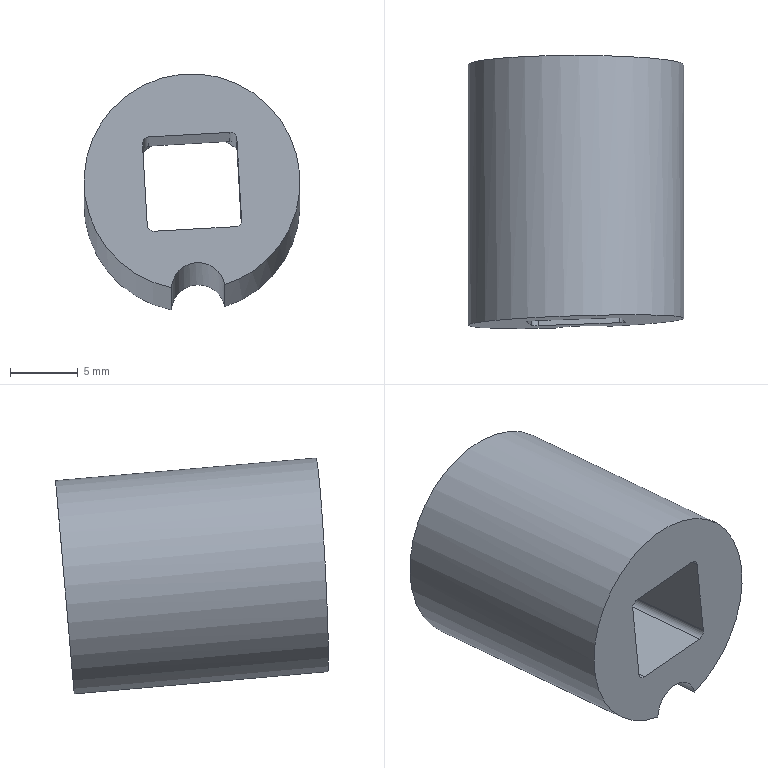Part | NX | features solid 2 | 1 solid | 14 faces | box 16 x 20.204 x 17.479 mm | volume 2341 mm3 | plane 7 | cylinder 7 | commonest cylinder face diameters 1 x4 4 x1 10.6 x1 16 x1
STEP:
#1=CARTESIAN_POINT('',(-229.897,-58.074,-39.843));
#2=VERTEX_POINT('',#1);
#3=CARTESIAN_POINT('',(-225.935,-57.934,-39.624));
#4=VERTEX_POINT('',#3);
#5=CARTESIAN_POINT('',(-227.901,-58.017,-39.983));
#6=DIRECTION('',(-0.03252,0.9981,-0.05307));
#7=DIRECTION('',(0.6892,-0.01607,-0.7244));
#8=AXIS2_PLACEMENT_3D('',#5,#6,#7);
#9=ELLIPSE('',#8,2.002,2.);
#10=EDGE_CURVE('',#2,#4,#9,.T.);
#11=ORIENTED_EDGE('',*,*,#10,.T.);
#12=CARTESIAN_POINT('',(-228.366,-57.608,-32.002));
#13=DIRECTION('',(-0.03252,0.9981,-0.05307));
#14=DIRECTION('',(0.6892,-0.01607,-0.7244));
#15=AXIS2_PLACEMENT_3D('',#12,#13,#14);
#16=ELLIPSE('',#15,8.009,8.);
#17=EDGE_CURVE('',#2,#4,#16,.T.);
#18=ORIENTED_EDGE('',*,*,#17,.F.);
#19=EDGE_LOOP('',(#11,#18));
#20=FACE_BOUND('',#19,.T.);
#21=CARTESIAN_POINT('',(-231.158,-57.893,-35.659));
#22=VERTEX_POINT('',#21);
#23=CARTESIAN_POINT('',(-225.168,-57.68,-35.328));
#24=VERTEX_POINT('',#23);
#25=CARTESIAN_POINT('',(-414.975,-64.423,-45.84));
#26=DIRECTION('',(-0.9978,-0.03545,-0.05527));
#27=VECTOR('',#26,1000.);
#28=LINE('',#25,#27);
#29=EDGE_CURVE('',#22,#24,#28,.F.);
#30=ORIENTED_EDGE('',*,*,#29,.F.);
#31=CARTESIAN_POINT('',(-231.686,-57.885,-35.188));
#32=VERTEX_POINT('',#31);
#33=CARTESIAN_POINT('',(-231.187,-57.867,-35.161));
#34=DIRECTION('',(-0.03252,0.9981,-0.05307));
#35=DIRECTION('',(-0.6892,0.01607,0.7244));
#36=AXIS2_PLACEMENT_3D('',#33,#34,#35);
#37=ELLIPSE('',#36,0.5006,0.5);
#38=EDGE_CURVE('',#22,#32,#37,.T.);
#39=ORIENTED_EDGE('',*,*,#38,.T.);
#40=CARTESIAN_POINT('',(-232.035,-57.578,-29.202));
#41=VERTEX_POINT('',#40);
#42=CARTESIAN_POINT('',(-239.027,-51.43,90.7));
#43=DIRECTION('',(0.05814,-0.05112,-0.997));
#44=VECTOR('',#43,1000.);
#45=LINE('',#42,#44);
#46=EDGE_CURVE('',#32,#41,#45,.F.);
#47=ORIENTED_EDGE('',*,*,#46,.T.);
#48=CARTESIAN_POINT('',(-231.565,-57.535,-28.676));
#49=VERTEX_POINT('',#48);
#50=CARTESIAN_POINT('',(-231.536,-57.561,-29.175));
#51=DIRECTION('',(-0.03252,0.9981,-0.05307));
#52=DIRECTION('',(0.6892,-0.01607,-0.7244));
#53=AXIS2_PLACEMENT_3D('',#50,#51,#52);
#54=ELLIPSE('',#53,0.5006,0.5);
#55=EDGE_CURVE('',#41,#49,#54,.T.);
#56=ORIENTED_EDGE('',*,*,#55,.T.);
#57=CARTESIAN_POINT('',(-225.575,-57.322,-28.344));
#58=VERTEX_POINT('',#57);
#59=CARTESIAN_POINT('',(-415.374,-64.065,-38.856));
#60=DIRECTION('',(-0.9978,-0.03545,-0.05527));
#61=VECTOR('',#60,1000.);
#62=LINE('',#59,#61);
#63=EDGE_CURVE('',#49,#58,#62,.F.);
#64=ORIENTED_EDGE('',*,*,#63,.T.);
#65=CARTESIAN_POINT('',(-225.047,-57.33,-28.815));
#66=VERTEX_POINT('',#65);
#67=CARTESIAN_POINT('',(-225.546,-57.348,-28.843));
#68=DIRECTION('',(-0.03252,0.9981,-0.05307));
#69=DIRECTION('',(0.6892,-0.01607,-0.7244));
#70=AXIS2_PLACEMENT_3D('',#67,#68,#69);
#71=ELLIPSE('',#70,0.5006,0.5);
#72=EDGE_CURVE('',#58,#66,#71,.T.);
#73=ORIENTED_EDGE('',*,*,#72,.T.);
#74=CARTESIAN_POINT('',(-224.698,-57.637,-34.801));
#75=VERTEX_POINT('',#74);
#76=CARTESIAN_POINT('',(-232.039,-51.182,91.094));
#77=DIRECTION('',(-0.05814,0.05112,0.997));
#78=VECTOR('',#77,1000.);
#79=LINE('',#76,#78);
#80=EDGE_CURVE('',#66,#75,#79,.F.);
#81=ORIENTED_EDGE('',*,*,#80,.T.);
#82=CARTESIAN_POINT('',(-225.197,-57.655,-34.829));
#83=DIRECTION('',(-0.03252,0.9981,-0.05307));
#84=DIRECTION('',(-0.6892,0.01607,0.7244));
#85=AXIS2_PLACEMENT_3D('',#82,#83,#84);
#86=ELLIPSE('',#85,0.5006,0.5);
#87=EDGE_CURVE('',#75,#24,#86,.T.);
#88=ORIENTED_EDGE('',*,*,#87,.T.);
#89=EDGE_LOOP('',(#30,#39,#47,#56,#64,#73,#81,#88));
#90=FACE_BOUND('',#89,.T.);
#91=CARTESIAN_POINT('',(-422.194,-57.948,80.353));
#92=DIRECTION('',(-0.03252,0.9981,-0.05307));
#93=DIRECTION('',(0.05223,-0.05133,-0.9973));
#94=AXIS2_PLACEMENT_3D('',#91,#92,#93);
#95=PLANE('',#94);
#96=ADVANCED_FACE('',(#20,#90),#95,.F.);
#97=CARTESIAN_POINT('',(-225.935,-39.263,-41.257));
#98=VERTEX_POINT('',#97);
#99=CARTESIAN_POINT('',(-229.897,-39.284,-41.487));
#100=VERTEX_POINT('',#99);
#101=CARTESIAN_POINT('',(-227.901,-39.295,-41.621));
#102=DIRECTION('',(0.,-0.9962,0.08716));
#103=DIRECTION('',(0.,-0.08716,-0.9962));
#104=AXIS2_PLACEMENT_3D('',#101,#102,#103);
#105=CIRCLE('',#104,2.);
#106=EDGE_CURVE('',#98,#100,#105,.T.);
#107=ORIENTED_EDGE('',*,*,#106,.T.);
#108=CARTESIAN_POINT('',(-228.366,-38.599,-33.665));
#109=DIRECTION('',(0.,-0.9962,0.08716));
#110=DIRECTION('',(0.,-0.08716,-0.9962));
#111=AXIS2_PLACEMENT_3D('',#108,#109,#110);
#112=CIRCLE('',#111,8.);
#113=EDGE_CURVE('',#98,#100,#112,.T.);
#114=ORIENTED_EDGE('',*,*,#113,.F.);
#115=EDGE_LOOP('',(#107,#114));
#116=FACE_BOUND('',#115,.T.);
#117=CARTESIAN_POINT('',(-228.366,-39.061,-38.945));
#118=VERTEX_POINT('',#117);
#119=CARTESIAN_POINT('',(-228.366,-38.599,-33.665));
#120=DIRECTION('',(0.,-0.9962,0.08716));
#121=DIRECTION('',(0.,-0.08716,-0.9962));
#122=AXIS2_PLACEMENT_3D('',#119,#120,#121);
#123=CIRCLE('',#122,5.3);
#124=EDGE_CURVE('',#118,#118,#123,.F.);
#125=ORIENTED_EDGE('',*,*,#124,.F.);
#126=EDGE_LOOP('',(#125));
#127=FACE_BOUND('',#126,.T.);
#128=CARTESIAN_POINT('',(-228.366,-38.62,-33.907));
#129=DIRECTION('',(0.,-0.9962,0.08716));
#130=DIRECTION('',(0.,-0.08716,-0.9962));
#131=AXIS2_PLACEMENT_3D('',#128,#129,#130);
#132=PLANE('',#131);
#133=ADVANCED_FACE('',(#116,#127),#132,.F.);
#134=CARTESIAN_POINT('',(-229.897,-48.729,-40.661));
#135=DIRECTION('',(0.,0.9962,-0.08716));
#136=VECTOR('',#135,1000.);
#137=LINE('',#134,#136);
#138=EDGE_CURVE('',#2,#100,#137,.T.);
#139=ORIENTED_EDGE('',*,*,#138,.F.);
#140=ORIENTED_EDGE('',*,*,#17,.T.);
#141=CARTESIAN_POINT('',(-225.935,-48.708,-40.431));
#142=DIRECTION('',(0.,0.9962,-0.08716));
#143=VECTOR('',#142,1000.);
#144=LINE('',#141,#143);
#145=EDGE_CURVE('',#98,#4,#144,.F.);
#146=ORIENTED_EDGE('',*,*,#145,.F.);
#147=ORIENTED_EDGE('',*,*,#113,.T.);
#148=EDGE_LOOP('',(#139,#140,#146,#147));
#149=FACE_BOUND('',#148,.T.);
#150=CARTESIAN_POINT('',(-228.366,-58.006,-31.967));
#151=DIRECTION('',(0.,0.9962,-0.08716));
#152=DIRECTION('',(-0.9997,-0.001977,-0.0226));
#153=AXIS2_PLACEMENT_3D('',#150,#151,#152);
#154=CYLINDRICAL_SURFACE('',#153,8.);
#155=ADVANCED_FACE('',(#149),#154,.T.);
#156=ORIENTED_EDGE('',*,*,#46,.F.);
#157=CARTESIAN_POINT('',(-231.686,-50.315,-35.85));
#158=VERTEX_POINT('',#157);
#159=CARTESIAN_POINT('',(-231.686,-65.756,-34.5));
#160=DIRECTION('',(0.,-0.9962,0.08716));
#161=VECTOR('',#160,1000.);
#162=LINE('',#159,#161);
#163=EDGE_CURVE('',#32,#158,#162,.F.);
#164=ORIENTED_EDGE('',*,*,#163,.T.);
#165=CARTESIAN_POINT('',(-232.035,-49.793,-29.883));
#166=VERTEX_POINT('',#165);
#167=CARTESIAN_POINT('',(-232.064,-49.75,-29.386));
#168=DIRECTION('',(0.05817,-0.08701,-0.9945));
#169=VECTOR('',#168,1000.);
#170=LINE('',#167,#169);
#171=EDGE_CURVE('',#166,#158,#170,.T.);
#172=ORIENTED_EDGE('',*,*,#171,.F.);
#173=CARTESIAN_POINT('',(-232.035,-65.234,-28.533));
#174=DIRECTION('',(0.,-0.9962,0.08716));
#175=VECTOR('',#174,1000.);
#176=LINE('',#173,#175);
#177=EDGE_CURVE('',#166,#41,#176,.T.);
#178=ORIENTED_EDGE('',*,*,#177,.T.);
#179=EDGE_LOOP('',(#156,#164,#172,#178));
#180=FACE_BOUND('',#179,.T.);
#181=CARTESIAN_POINT('',(-232.064,-65.191,-28.035));
#182=DIRECTION('',(0.9983,0.00507,0.05795));
#183=DIRECTION('',(-0.05817,0.08701,0.9945));
#184=AXIS2_PLACEMENT_3D('',#181,#182,#183);
#185=PLANE('',#184);
#186=ADVANCED_FACE('',(#180),#185,.T.);
#187=CARTESIAN_POINT('',(-225.168,-50.326,-35.971));
#188=VERTEX_POINT('',#187);
#189=CARTESIAN_POINT('',(-231.158,-50.356,-36.319));
#190=VERTEX_POINT('',#189);
#191=CARTESIAN_POINT('',(-224.669,-50.323,-35.942));
#192=DIRECTION('',(-0.9983,-0.00507,-0.05795));
#193=VECTOR('',#192,1000.);
#194=LINE('',#191,#193);
#195=EDGE_CURVE('',#188,#190,#194,.T.);
#196=ORIENTED_EDGE('',*,*,#195,.T.);
#197=CARTESIAN_POINT('',(-231.158,-65.797,-34.968));
#198=DIRECTION('',(0.,-0.9962,0.08716));
#199=VECTOR('',#198,1000.);
#200=LINE('',#197,#199);
#201=EDGE_CURVE('',#190,#22,#200,.T.);
#202=ORIENTED_EDGE('',*,*,#201,.T.);
#203=ORIENTED_EDGE('',*,*,#29,.T.);
#204=CARTESIAN_POINT('',(-225.168,-65.767,-34.62));
#205=DIRECTION('',(0.,-0.9962,0.08716));
#206=VECTOR('',#205,1000.);
#207=LINE('',#204,#206);
#208=EDGE_CURVE('',#24,#188,#207,.F.);
#209=ORIENTED_EDGE('',*,*,#208,.T.);
#210=EDGE_LOOP('',(#196,#202,#203,#209));
#211=FACE_BOUND('',#210,.T.);
#212=CARTESIAN_POINT('',(-224.669,-65.764,-34.591));
#213=DIRECTION('',(0.05817,-0.08701,-0.9945));
#214=DIRECTION('',(0.9983,0.00507,0.05795));
#215=AXIS2_PLACEMENT_3D('',#212,#213,#214);
#216=PLANE('',#215);
#217=ADVANCED_FACE('',(#211),#216,.F.);
#218=CARTESIAN_POINT('',(-224.698,-50.28,-35.445));
#219=VERTEX_POINT('',#218);
#220=CARTESIAN_POINT('',(-225.047,-49.758,-29.478));
#221=VERTEX_POINT('',#220);
#222=CARTESIAN_POINT('',(-224.669,-50.323,-35.942));
#223=DIRECTION('',(-0.05817,0.08701,0.9945));
#224=VECTOR('',#223,1000.);
#225=LINE('',#222,#224);
#226=EDGE_CURVE('',#219,#221,#225,.T.);
#227=ORIENTED_EDGE('',*,*,#226,.F.);
#228=CARTESIAN_POINT('',(-224.698,-65.721,-34.094));
#229=DIRECTION('',(0.,-0.9962,0.08716));
#230=VECTOR('',#229,1000.);
#231=LINE('',#228,#230);
#232=EDGE_CURVE('',#219,#75,#231,.T.);
#233=ORIENTED_EDGE('',*,*,#232,.T.);
#234=ORIENTED_EDGE('',*,*,#80,.F.);
#235=CARTESIAN_POINT('',(-225.047,-65.199,-28.127));
#236=DIRECTION('',(0.,-0.9962,0.08716));
#237=VECTOR('',#236,1000.);
#238=LINE('',#235,#237);
#239=EDGE_CURVE('',#66,#221,#238,.F.);
#240=ORIENTED_EDGE('',*,*,#239,.T.);
#241=EDGE_LOOP('',(#227,#233,#234,#240));
#242=FACE_BOUND('',#241,.T.);
#243=CARTESIAN_POINT('',(-224.669,-65.764,-34.591));
#244=DIRECTION('',(-0.9983,-0.00507,-0.05795));
#245=DIRECTION('',(0.05817,-0.08701,-0.9945));
#246=AXIS2_PLACEMENT_3D('',#243,#244,#245);
#247=PLANE('',#246);
#248=ADVANCED_FACE('',(#242),#247,.T.);
#249=ORIENTED_EDGE('',*,*,#63,.F.);
#250=CARTESIAN_POINT('',(-231.565,-49.747,-29.357));
#251=VERTEX_POINT('',#250);
#252=CARTESIAN_POINT('',(-231.565,-65.188,-28.006));
#253=DIRECTION('',(0.,-0.9962,0.08716));
#254=VECTOR('',#253,1000.);
#255=LINE('',#252,#254);
#256=EDGE_CURVE('',#49,#251,#255,.F.);
#257=ORIENTED_EDGE('',*,*,#256,.T.);
#258=CARTESIAN_POINT('',(-225.575,-49.717,-29.009));
#259=VERTEX_POINT('',#258);
#260=CARTESIAN_POINT('',(-225.076,-49.714,-28.98));
#261=DIRECTION('',(-0.9983,-0.00507,-0.05795));
#262=VECTOR('',#261,1000.);
#263=LINE('',#260,#262);
#264=EDGE_CURVE('',#259,#251,#263,.T.);
#265=ORIENTED_EDGE('',*,*,#264,.F.);
#266=CARTESIAN_POINT('',(-225.575,-65.158,-27.659));
#267=DIRECTION('',(0.,-0.9962,0.08716));
#268=VECTOR('',#267,1000.);
#269=LINE('',#266,#268);
#270=EDGE_CURVE('',#259,#58,#269,.T.);
#271=ORIENTED_EDGE('',*,*,#270,.T.);
#272=EDGE_LOOP('',(#249,#257,#265,#271));
#273=FACE_BOUND('',#272,.T.);
#274=CARTESIAN_POINT('',(-225.076,-65.155,-27.63));
#275=DIRECTION('',(0.05817,-0.08701,-0.9945));
#276=DIRECTION('',(0.9983,0.00507,0.05795));
#277=AXIS2_PLACEMENT_3D('',#274,#275,#276);
#278=PLANE('',#277);
#279=ADVANCED_FACE('',(#273),#278,.T.);
#280=ORIENTED_EDGE('',*,*,#264,.T.);
#281=CARTESIAN_POINT('',(-231.536,-49.791,-29.854));
#282=DIRECTION('',(0.,-0.9962,0.08716));
#283=DIRECTION('',(0.,-0.08716,-0.9962));
#284=AXIS2_PLACEMENT_3D('',#281,#282,#283);
#285=CIRCLE('',#284,0.5);
#286=EDGE_CURVE('',#251,#166,#285,.T.);
#287=ORIENTED_EDGE('',*,*,#286,.T.);
#288=ORIENTED_EDGE('',*,*,#171,.T.);
#289=CARTESIAN_POINT('',(-231.187,-50.313,-35.821));
#290=DIRECTION('',(0.,-0.9962,0.08716));
#291=DIRECTION('',(0.,-0.08716,-0.9962));
#292=AXIS2_PLACEMENT_3D('',#289,#290,#291);
#293=CIRCLE('',#292,0.5);
#294=EDGE_CURVE('',#158,#190,#293,.T.);
#295=ORIENTED_EDGE('',*,*,#294,.T.);
#296=ORIENTED_EDGE('',*,*,#195,.F.);
#297=CARTESIAN_POINT('',(-225.197,-50.282,-35.474));
#298=DIRECTION('',(0.,-0.9962,0.08716));
#299=DIRECTION('',(0.,-0.08716,-0.9962));
#300=AXIS2_PLACEMENT_3D('',#297,#298,#299);
#301=CIRCLE('',#300,0.5);
#302=EDGE_CURVE('',#188,#219,#301,.T.);
#303=ORIENTED_EDGE('',*,*,#302,.T.);
#304=ORIENTED_EDGE('',*,*,#226,.T.);
#305=CARTESIAN_POINT('',(-225.546,-49.76,-29.507));
#306=DIRECTION('',(0.,-0.9962,0.08716));
#307=DIRECTION('',(0.,-0.08716,-0.9962));
#308=AXIS2_PLACEMENT_3D('',#305,#306,#307);
#309=CIRCLE('',#308,0.5);
#310=EDGE_CURVE('',#221,#259,#309,.T.);
#311=ORIENTED_EDGE('',*,*,#310,.T.);
#312=EDGE_LOOP('',(#280,#287,#288,#295,#296,#303,#304,#311));
#313=FACE_BOUND('',#312,.T.);
#314=CARTESIAN_POINT('',(-233.665,-50.047,-32.784));
#315=VERTEX_POINT('',#314);
#316=CARTESIAN_POINT('',(-228.366,-50.037,-32.664));
#317=DIRECTION('',(0.,0.9962,-0.08716));
#318=DIRECTION('',(-0.9997,-0.001977,-0.0226));
#319=AXIS2_PLACEMENT_3D('',#316,#317,#318);
#320=CIRCLE('',#319,5.3);
#321=EDGE_CURVE('',#315,#315,#320,.T.);
#322=ORIENTED_EDGE('',*,*,#321,.T.);
#323=EDGE_LOOP('',(#322));
#324=FACE_BOUND('',#323,.T.);
#325=CARTESIAN_POINT('',(-228.366,-50.037,-32.664));
#326=DIRECTION('',(0.,-0.9962,0.08716));
#327=DIRECTION('',(0.9997,0.001977,0.0226));
#328=AXIS2_PLACEMENT_3D('',#325,#326,#327);
#329=PLANE('',#328);
#330=ADVANCED_FACE('',(#313,#324),#329,.F.);
#331=ORIENTED_EDGE('',*,*,#124,.T.);
#332=EDGE_LOOP('',(#331));
#333=FACE_BOUND('',#332,.T.);
#334=ORIENTED_EDGE('',*,*,#321,.F.);
#335=EDGE_LOOP('',(#334));
#336=FACE_BOUND('',#335,.T.);
#337=CARTESIAN_POINT('',(-228.366,-50.037,-32.664));
#338=DIRECTION('',(0.,0.9962,-0.08716));
#339=DIRECTION('',(-0.9997,-0.001977,-0.0226));
#340=AXIS2_PLACEMENT_3D('',#337,#338,#339);
#341=CYLINDRICAL_SURFACE('',#340,5.3);
#342=ADVANCED_FACE('',(#333,#336),#341,.F.);
#343=ORIENTED_EDGE('',*,*,#138,.T.);
#344=ORIENTED_EDGE('',*,*,#106,.F.);
#345=ORIENTED_EDGE('',*,*,#145,.T.);
#346=ORIENTED_EDGE('',*,*,#10,.F.);
#347=EDGE_LOOP('',(#343,#344,#345,#346));
#348=FACE_BOUND('',#347,.T.);
#349=CARTESIAN_POINT('',(-227.901,-58.702,-39.923));
#350=DIRECTION('',(0.,0.9962,-0.08716));
#351=DIRECTION('',(-0.9997,-0.001977,-0.0226));
#352=AXIS2_PLACEMENT_3D('',#349,#350,#351);
#353=CYLINDRICAL_SURFACE('',#352,2.);
#354=ADVANCED_FACE('',(#348),#353,.F.);
#355=ORIENTED_EDGE('',*,*,#38,.F.);
#356=ORIENTED_EDGE('',*,*,#201,.F.);
#357=ORIENTED_EDGE('',*,*,#294,.F.);
#358=ORIENTED_EDGE('',*,*,#163,.F.);
#359=EDGE_LOOP('',(#355,#356,#357,#358));
#360=FACE_BOUND('',#359,.T.);
#361=CARTESIAN_POINT('',(-231.187,-65.754,-34.471));
#362=DIRECTION('',(0.,-0.9962,0.08716));
#363=DIRECTION('',(0.,-0.08716,-0.9962));
#364=AXIS2_PLACEMENT_3D('',#361,#362,#363);
#365=CYLINDRICAL_SURFACE('',#364,0.5);
#366=ADVANCED_FACE('',(#360),#365,.F.);
#367=ORIENTED_EDGE('',*,*,#87,.F.);
#368=ORIENTED_EDGE('',*,*,#232,.F.);
#369=ORIENTED_EDGE('',*,*,#302,.F.);
#370=ORIENTED_EDGE('',*,*,#208,.F.);
#371=EDGE_LOOP('',(#367,#368,#369,#370));
#372=FACE_BOUND('',#371,.T.);
#373=CARTESIAN_POINT('',(-225.197,-65.723,-34.123));
#374=DIRECTION('',(0.,-0.9962,0.08716));
#375=DIRECTION('',(0.,-0.08716,-0.9962));
#376=AXIS2_PLACEMENT_3D('',#373,#374,#375);
#377=CYLINDRICAL_SURFACE('',#376,0.5);
#378=ADVANCED_FACE('',(#372),#377,.F.);
#379=ORIENTED_EDGE('',*,*,#55,.F.);
#380=ORIENTED_EDGE('',*,*,#177,.F.);
#381=ORIENTED_EDGE('',*,*,#286,.F.);
#382=ORIENTED_EDGE('',*,*,#256,.F.);
#383=EDGE_LOOP('',(#379,#380,#381,#382));
#384=FACE_BOUND('',#383,.T.);
#385=CARTESIAN_POINT('',(-231.536,-65.232,-28.504));
#386=DIRECTION('',(0.,0.9962,-0.08716));
#387=DIRECTION('',(0.,0.08716,0.9962));
#388=AXIS2_PLACEMENT_3D('',#385,#386,#387);
#389=CYLINDRICAL_SURFACE('',#388,0.5);
#390=ADVANCED_FACE('',(#384),#389,.F.);
#391=ORIENTED_EDGE('',*,*,#72,.F.);
#392=ORIENTED_EDGE('',*,*,#270,.F.);
#393=ORIENTED_EDGE('',*,*,#310,.F.);
#394=ORIENTED_EDGE('',*,*,#239,.F.);
#395=EDGE_LOOP('',(#391,#392,#393,#394));
#396=FACE_BOUND('',#395,.T.);
#397=CARTESIAN_POINT('',(-225.546,-65.201,-28.156));
#398=DIRECTION('',(0.,0.9962,-0.08716));
#399=DIRECTION('',(0.,0.08716,0.9962));
#400=AXIS2_PLACEMENT_3D('',#397,#398,#399);
#401=CYLINDRICAL_SURFACE('',#400,0.5);
#402=ADVANCED_FACE('',(#396),#401,.F.);
#403=CLOSED_SHELL('',(#96,#133,#155,#186,#217,#248,#279,#330,#342,#354,#366,#378,#390,#402));
#404=MANIFOLD_SOLID_BREP('',#403);
#405=(LENGTH_UNIT()NAMED_UNIT(*)SI_UNIT(.MILLI.,.METRE.));
#406=UNCERTAINTY_MEASURE_WITH_UNIT(LENGTH_MEASURE(0.00001),#405,'','');
#407=(NAMED_UNIT(*)PLANE_ANGLE_UNIT()SI_UNIT($,.RADIAN.));
#408=(NAMED_UNIT(*)SI_UNIT($,.STERADIAN.)SOLID_ANGLE_UNIT());
#409=(GEOMETRIC_REPRESENTATION_CONTEXT(3)GLOBAL_UNCERTAINTY_ASSIGNED_CONTEXT((#406))GLOBAL_UNIT_ASSIGNED_CONTEXT((#405,#407,#408))REPRESENTATION_CONTEXT('',''));
#410=ADVANCED_BREP_SHAPE_REPRESENTATION('',(#404),#409);